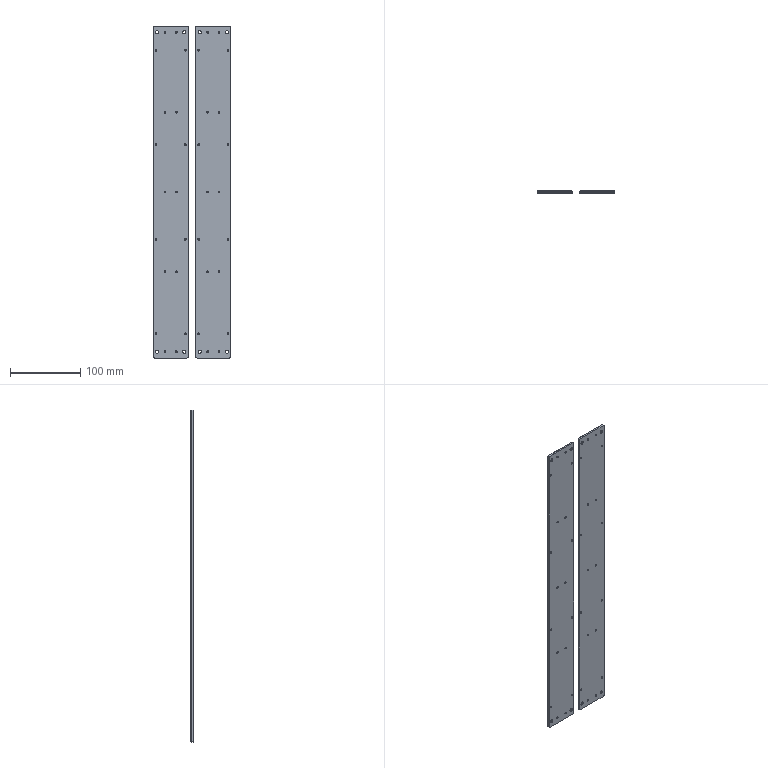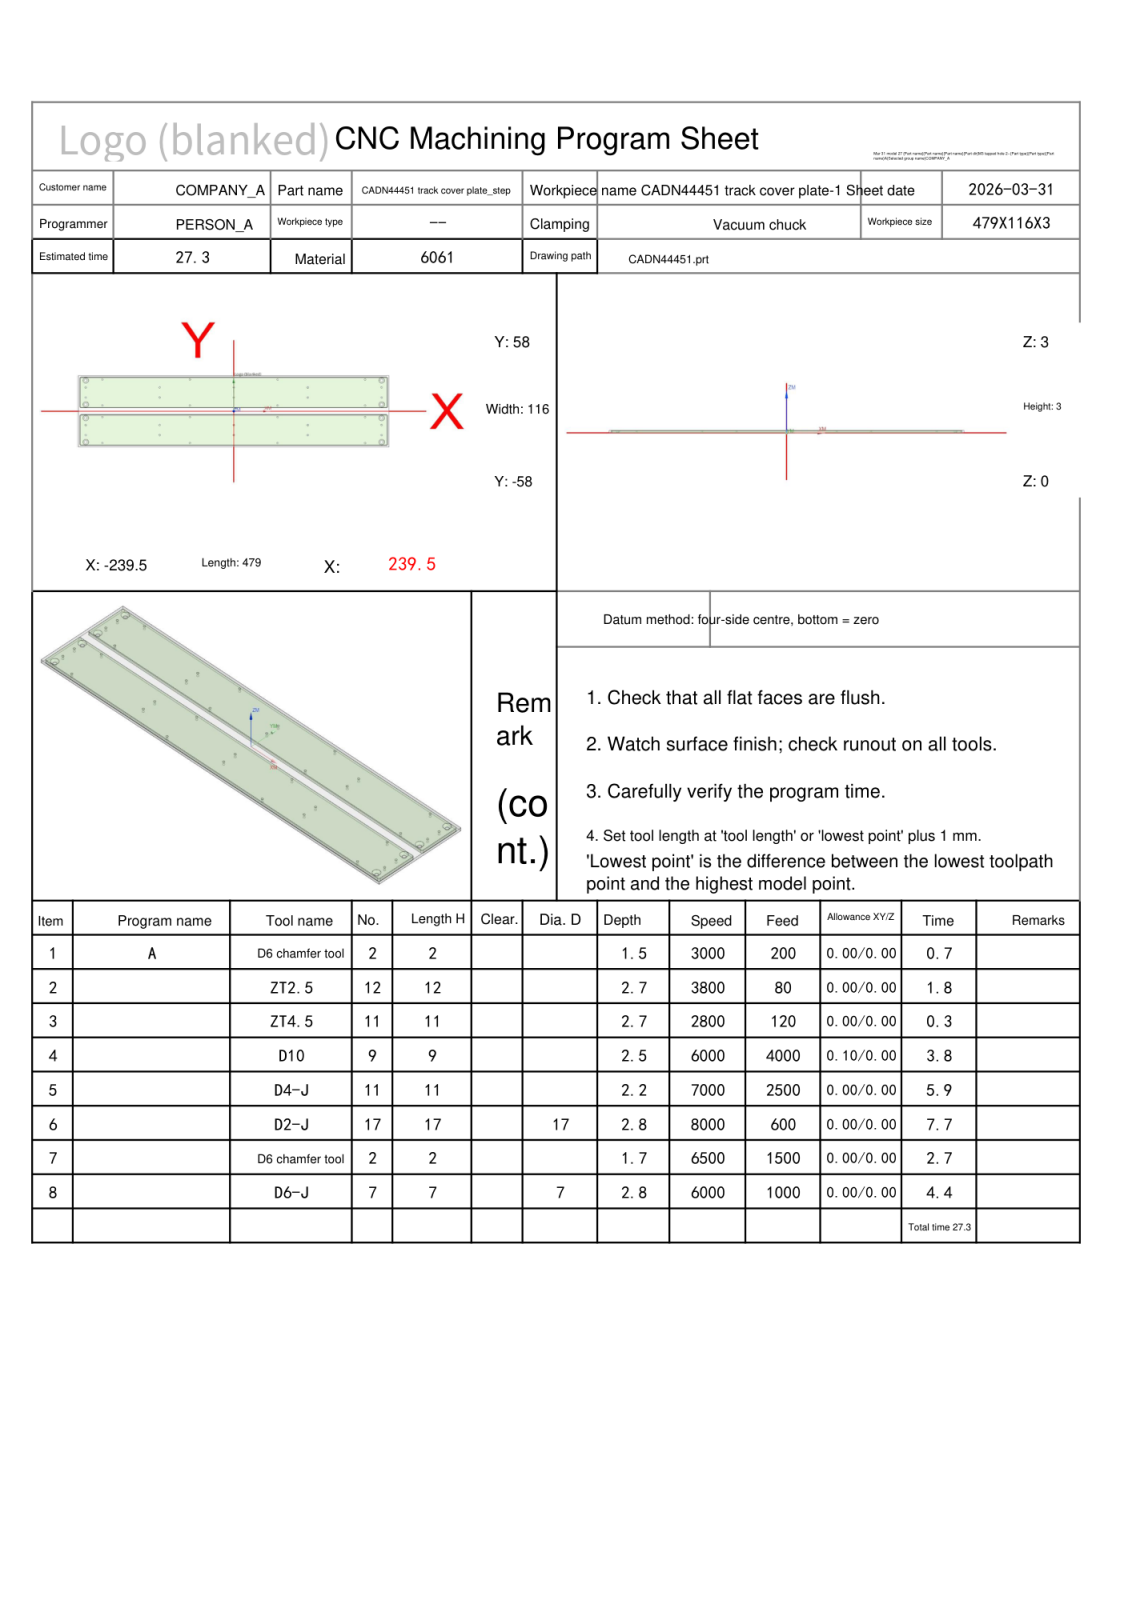NC program | NX | posted by the shop | part box 111 x 3 x 474 mm
Lines 11150 to 12144 of 17996:
N6 T17 M06
(D2-J  D=2. R=0. H=17 ce=0.00 di=0.00)
G00 G90 G54 X229.215 Y49.987 M03 S8000
G43 H17 Z23.
M08
Z1.5
G01 Y50.11 Z1.494 F600.
X229.159 Y50.381 Z1.479
X229.044 Y50.632 Z1.465
X228.875 Y50.85 Z1.45
X228.662 Y51.025 Z1.436
X228.414 Y51.148 Z1.421
X228.146 Y51.211 Z1.407
X227.89 Y51.215 Z1.393
X227.614 Y51.157 Z1.379
X227.358 Y51.038 Z1.364
X227.137 Y50.863 Z1.349
X226.962 Y50.642 Z1.334
X226.843 Y50.386 Z1.319
X226.785 Y50.11 Z1.305
Y49.89 Z1.293
X226.843 Y49.614 Z1.278
X226.962 Y49.358 Z1.264
X227.137 Y49.137 Z1.249
X227.358 Y48.962 Z1.234
X227.614 Y48.843 Z1.219
X227.89 Y48.785 Z1.204
X228.11 Z1.193
X228.386 Y48.843 Z1.178
X228.642 Y48.962 Z1.163
X228.863 Y49.137 Z1.148
X229.038 Y49.358 Z1.134
X229.157 Y49.614 Z1.119
X229.215 Y49.89 Z1.104
Y50.11 Z1.093
X229.159 Y50.381 Z1.078
X229.044 Y50.632 Z1.064
X228.875 Y50.85 Z1.049
X228.662 Y51.025 Z1.035
X228.414 Y51.148 Z1.02
X228.146 Y51.211 Z1.006
X228.035 Y51.215 Z1.
G41 D17
X228. Y51.25
G03 X226.75 Y50. Z.958 I0.0 J-1.25
X228. Y48.75 Z.915 I1.25 J0.0
X229.25 Y50. Z.873 I0.0 J1.25
X228. Y51.25 Z.83 I-1.25 J0.0
X226.75 Y50. Z.788 I0.0 J-1.25
X228. Y48.75 Z.745 I1.25 J0.0
X229.25 Y50. Z.703 I0.0 J1.25
X228. Y51.25 Z.66 I-1.25 J0.0
X226.75 Y50. Z.618 I0.0 J-1.25
X228. Y48.75 Z.575 I1.25 J0.0
X229.25 Y50. Z.533 I0.0 J1.25
X228. Y51.25 Z.49 I-1.25 J0.0
X226.75 Y50. Z.448 I0.0 J-1.25
X228. Y48.75 Z.405 I1.25 J0.0
X229.25 Y50. Z.363 I0.0 J1.25
X228. Y51.25 Z.32 I-1.25 J0.0
X226.75 Y50. Z.278 I0.0 J-1.25
X228. Y48.75 Z.235 I1.25 J0.0
X229.25 Y50. Z.193 I0.0 J1.25
X228. Y51.25 Z.15 I-1.25 J0.0
X226.75 Y50. I0.0 J-1.25
X228. Y48.75 I1.25 J0.0
X229.25 Y50. I0.0 J1.25
X228. Y51.25 I-1.25 J0.0
X227.607 Y51.187 I0.0 J-1.25
G01 X227.581 Y51.176
X227.569 Y51.15
X227.575 Y51.123
G40 X227.591 Y51.076
Z1.15
G00 Z23.
X227.987 Y9.785
Z1.5
G01 X228.11 Z1.494
X228.381 Y9.841 Z1.479
X228.632 Y9.956 Z1.465
X228.85 Y10.125 Z1.45
X229.025 Y10.338 Z1.436
X229.148 Y10.586 Z1.421
X229.211 Y10.854 Z1.407
X229.215 Y11.11 Z1.393
X229.157 Y11.386 Z1.379
X229.038 Y11.642 Z1.364
X228.863 Y11.863 Z1.349
X228.642 Y12.038 Z1.334
X228.386 Y12.157 Z1.319
X228.11 Y12.215 Z1.305
X227.89 Z1.293
X227.614 Y12.157 Z1.278
X227.358 Y12.038 Z1.264
X227.137 Y11.863 Z1.249
X226.962 Y11.642 Z1.234
X226.843 Y11.386 Z1.219
X226.785 Y11.11 Z1.204
Y10.89 Z1.193
X226.843 Y10.614 Z1.178
X226.962 Y10.358 Z1.163
X227.137 Y10.137 Z1.148
X227.358 Y9.962 Z1.134
X227.614 Y9.843 Z1.119
X227.89 Y9.785 Z1.104
X228.11 Z1.093
X228.381 Y9.841 Z1.078
X228.632 Y9.956 Z1.064
X228.85 Y10.125 Z1.049
X229.025 Y10.338 Z1.035
X229.148 Y10.586 Z1.02
X229.211 Y10.854 Z1.006
X229.215 Y10.965 Z1.
G41 D17
X229.25 Y11.
G03 X228. Y12.25 Z.958 I-1.25 J0.0
X226.75 Y11. Z.915 I0.0 J-1.25
X228. Y9.75 Z.873 I1.25 J0.0
X229.25 Y11. Z.83 I0.0 J1.25
X228. Y12.25 Z.788 I-1.25 J0.0
X226.75 Y11. Z.745 I0.0 J-1.25
X228. Y9.75 Z.703 I1.25 J0.0
X229.25 Y11. Z.66 I0.0 J1.25
X228. Y12.25 Z.618 I-1.25 J0.0
X226.75 Y11. Z.575 I0.0 J-1.25
X228. Y9.75 Z.533 I1.25 J0.0
X229.25 Y11. Z.49 I0.0 J1.25
X228. Y12.25 Z.448 I-1.25 J0.0
X226.75 Y11. Z.405 I0.0 J-1.25
X228. Y9.75 Z.363 I1.25 J0.0
X229.25 Y11. Z.32 I0.0 J1.25
X228. Y12.25 Z.278 I-1.25 J0.0
X226.75 Y11. Z.235 I0.0 J-1.25
X228. Y9.75 Z.193 I1.25 J0.0
X229.25 Y11. Z.15 I0.0 J1.25
X228. Y12.25 I-1.25 J0.0
X226.75 Y11. I0.0 J-1.25
X228. Y9.75 I1.25 J0.0
X229.25 Y11. I0.0 J1.25
X229.187 Y11.393 I-1.25 J0.0
G01 X229.176 Y11.419
X229.15 Y11.431
X229.123 Y11.425
G40 X229.076 Y11.409
Z1.15
G00 Z23.
X227.987 Y-12.215
Z1.5
G01 X228.11 Z1.494
X228.381 Y-12.159 Z1.479
X228.632 Y-12.044 Z1.465
X228.85 Y-11.875 Z1.45
X229.025 Y-11.662 Z1.436
X229.148 Y-11.414 Z1.421
X229.211 Y-11.146 Z1.407
X229.215 Y-10.89 Z1.393
X229.157 Y-10.614 Z1.379
X229.038 Y-10.358 Z1.364
X228.863 Y-10.137 Z1.349
X228.642 Y-9.962 Z1.334
X228.386 Y-9.843 Z1.319
X228.11 Y-9.785 Z1.305
X227.89 Z1.293
X227.614 Y-9.843 Z1.278
X227.358 Y-9.962 Z1.264
X227.137 Y-10.137 Z1.249
X226.962 Y-10.358 Z1.234
X226.843 Y-10.614 Z1.219
X226.785 Y-10.89 Z1.204
Y-11.11 Z1.193
X226.843 Y-11.386 Z1.178
X226.962 Y-11.642 Z1.163
X227.137 Y-11.863 Z1.148
X227.358 Y-12.038 Z1.134
X227.614 Y-12.157 Z1.119
X227.89 Y-12.215 Z1.104
X228.11 Z1.093
X228.381 Y-12.159 Z1.078
X228.632 Y-12.044 Z1.064
X228.85 Y-11.875 Z1.049
X229.025 Y-11.662 Z1.035
X229.148 Y-11.414 Z1.02
X229.211 Y-11.146 Z1.006
X229.215 Y-11.035 Z1.
G41 D17
X229.25 Y-11.
G03 X228. Y-9.75 Z.958 I-1.25 J0.0
X226.75 Y-11. Z.915 I0.0 J-1.25
X228. Y-12.25 Z.873 I1.25 J0.0
X229.25 Y-11. Z.83 I0.0 J1.25
X228. Y-9.75 Z.788 I-1.25 J0.0
X226.75 Y-11. Z.745 I0.0 J-1.25
X228. Y-12.25 Z.703 I1.25 J0.0
X229.25 Y-11. Z.66 I0.0 J1.25
X228. Y-9.75 Z.618 I-1.25 J0.0
X226.75 Y-11. Z.575 I0.0 J-1.25
X228. Y-12.25 Z.533 I1.25 J0.0
X229.25 Y-11. Z.49 I0.0 J1.25
X228. Y-9.75 Z.448 I-1.25 J0.0
X226.75 Y-11. Z.405 I0.0 J-1.25
X228. Y-12.25 Z.363 I1.25 J0.0
X229.25 Y-11. Z.32 I0.0 J1.25
X228. Y-9.75 Z.278 I-1.25 J0.0
X226.75 Y-11. Z.235 I0.0 J-1.25
X228. Y-12.25 Z.193 I1.25 J0.0
X229.25 Y-11. Z.15 I0.0 J1.25
X228. Y-9.75 I-1.25 J0.0
X226.75 Y-11. I0.0 J-1.25
X228. Y-12.25 I1.25 J0.0
X229.25 Y-11. I0.0 J1.25
X229.187 Y-10.607 I-1.25 J0.0
G01 X229.176 Y-10.581
X229.15 Y-10.569
X229.123 Y-10.575
G40 X229.076 Y-10.591
Z1.15
G00 Z23.
X226.785 Y-49.987
Z1.5
G01 Y-50.11 Z1.494
X226.841 Y-50.381 Z1.479
X226.956 Y-50.632 Z1.465
X227.125 Y-50.85 Z1.45
X227.338 Y-51.025 Z1.436
X227.586 Y-51.148 Z1.421
X227.854 Y-51.211 Z1.407
X228.11 Y-51.215 Z1.393
X228.386 Y-51.157 Z1.379
X228.642 Y-51.038 Z1.364
X228.863 Y-50.863 Z1.349
X229.038 Y-50.642 Z1.334
X229.157 Y-50.386 Z1.319
X229.215 Y-50.11 Z1.305
Y-49.89 Z1.293
X229.157 Y-49.614 Z1.278
X229.038 Y-49.358 Z1.264
X228.863 Y-49.137 Z1.249
X228.642 Y-48.962 Z1.234
X228.386 Y-48.843 Z1.219
X228.11 Y-48.785 Z1.204
X227.89 Z1.193
X227.614 Y-48.843 Z1.178
X227.358 Y-48.962 Z1.163
X227.137 Y-49.137 Z1.148
X226.962 Y-49.358 Z1.134
X226.843 Y-49.614 Z1.119
X226.785 Y-49.89 Z1.104
Y-50.11 Z1.093
X226.841 Y-50.381 Z1.078
X226.956 Y-50.632 Z1.064
X227.125 Y-50.85 Z1.049
X227.338 Y-51.025 Z1.035
X227.586 Y-51.148 Z1.02
X227.854 Y-51.211 Z1.006
X227.965 Y-51.215 Z1.
G41 D17
X228. Y-51.25
G03 X229.25 Y-50. Z.958 I0.0 J1.25
X228. Y-48.75 Z.915 I-1.25 J0.0
X226.75 Y-50. Z.873 I0.0 J-1.25
X228. Y-51.25 Z.83 I1.25 J0.0
X229.25 Y-50. Z.788 I0.0 J1.25
X228. Y-48.75 Z.745 I-1.25 J0.0
X226.75 Y-50. Z.703 I0.0 J-1.25
X228. Y-51.25 Z.66 I1.25 J0.0
X229.25 Y-50. Z.618 I0.0 J1.25
X228. Y-48.75 Z.575 I-1.25 J0.0
X226.75 Y-50. Z.533 I0.0 J-1.25
X228. Y-51.25 Z.49 I1.25 J0.0
X229.25 Y-50. Z.448 I0.0 J1.25
X228. Y-48.75 Z.405 I-1.25 J0.0
X226.75 Y-50. Z.363 I0.0 J-1.25
X228. Y-51.25 Z.32 I1.25 J0.0
X229.25 Y-50. Z.278 I0.0 J1.25
X228. Y-48.75 Z.235 I-1.25 J0.0
X226.75 Y-50. Z.193 I0.0 J-1.25
X228. Y-51.25 Z.15 I1.25 J0.0
X229.25 Y-50. I0.0 J1.25
X228. Y-48.75 I-1.25 J0.0
X226.75 Y-50. I0.0 J-1.25
X228. Y-51.25 I1.25 J0.0
X228.393 Y-51.187 I0.0 J1.25
G01 X228.419 Y-51.176
X228.431 Y-51.15
X228.425 Y-51.123
G40 X228.409 Y-51.076
Z1.15
G00 Z23.
X-229.215 Y-49.987
Z1.5
G01 Y-50.11 Z1.494
X-229.159 Y-50.381 Z1.479
X-229.044 Y-50.632 Z1.465
X-228.875 Y-50.85 Z1.45
X-228.662 Y-51.025 Z1.436
X-228.414 Y-51.148 Z1.421
X-228.146 Y-51.211 Z1.407
X-227.89 Y-51.215 Z1.393
X-227.614 Y-51.157 Z1.379
X-227.358 Y-51.038 Z1.364
X-227.137 Y-50.863 Z1.349
X-226.962 Y-50.642 Z1.334
X-226.843 Y-50.386 Z1.319
X-226.785 Y-50.11 Z1.305
Y-49.89 Z1.293
X-226.843 Y-49.614 Z1.278
X-226.962 Y-49.358 Z1.264
X-227.137 Y-49.137 Z1.249
X-227.358 Y-48.962 Z1.234
X-227.614 Y-48.843 Z1.219
X-227.89 Y-48.785 Z1.204
X-228.11 Z1.193
X-228.386 Y-48.843 Z1.178
X-228.642 Y-48.962 Z1.163
X-228.863 Y-49.137 Z1.148
X-229.038 Y-49.358 Z1.134
X-229.157 Y-49.614 Z1.119
X-229.215 Y-49.89 Z1.104
Y-50.11 Z1.093
X-229.159 Y-50.381 Z1.078
X-229.044 Y-50.632 Z1.064
X-228.875 Y-50.85 Z1.049
X-228.662 Y-51.025 Z1.035
X-228.414 Y-51.148 Z1.02
X-228.146 Y-51.211 Z1.006
X-228.035 Y-51.215 Z1.
G41 D17
X-228. Y-51.25
G03 X-226.75 Y-50. Z.958 I0.0 J1.25
X-228. Y-48.75 Z.915 I-1.25 J0.0
X-229.25 Y-50. Z.873 I0.0 J-1.25
X-228. Y-51.25 Z.83 I1.25 J0.0
X-226.75 Y-50. Z.788 I0.0 J1.25
X-228. Y-48.75 Z.745 I-1.25 J0.0
X-229.25 Y-50. Z.703 I0.0 J-1.25
X-228. Y-51.25 Z.66 I1.25 J0.0
X-226.75 Y-50. Z.618 I0.0 J1.25
X-228. Y-48.75 Z.575 I-1.25 J0.0
X-229.25 Y-50. Z.533 I0.0 J-1.25
X-228. Y-51.25 Z.49 I1.25 J0.0
X-226.75 Y-50. Z.448 I0.0 J1.25
X-228. Y-48.75 Z.405 I-1.25 J0.0
X-229.25 Y-50. Z.363 I0.0 J-1.25
X-228. Y-51.25 Z.32 I1.25 J0.0
X-226.75 Y-50. Z.278 I0.0 J1.25
X-228. Y-48.75 Z.235 I-1.25 J0.0
X-229.25 Y-50. Z.193 I0.0 J-1.25
X-228. Y-51.25 Z.15 I1.25 J0.0
X-226.75 Y-50. I0.0 J1.25
X-228. Y-48.75 I-1.25 J0.0
X-229.25 Y-50. I0.0 J-1.25
X-228. Y-51.25 I1.25 J0.0
X-227.607 Y-51.187 I0.0 J1.25
G01 X-227.581 Y-51.176
X-227.569 Y-51.15
X-227.575 Y-51.123
G40 X-227.591 Y-51.076
Z1.15
G00 Z23.
X-227.987 Y-9.785
Z1.5
G01 X-228.11 Z1.494
X-228.381 Y-9.841 Z1.479
X-228.632 Y-9.956 Z1.465
X-228.85 Y-10.125 Z1.45
X-229.025 Y-10.338 Z1.436
X-229.148 Y-10.586 Z1.421
X-229.211 Y-10.854 Z1.407
X-229.215 Y-11.11 Z1.393
X-229.157 Y-11.386 Z1.379
X-229.038 Y-11.642 Z1.364
X-228.863 Y-11.863 Z1.349
X-228.642 Y-12.038 Z1.334
X-228.386 Y-12.157 Z1.319
X-228.11 Y-12.215 Z1.305
X-227.89 Z1.293
X-227.614 Y-12.157 Z1.278
X-227.358 Y-12.038 Z1.264
X-227.137 Y-11.863 Z1.249
X-226.962 Y-11.642 Z1.234
X-226.843 Y-11.386 Z1.219
X-226.785 Y-11.11 Z1.204
Y-10.89 Z1.193
X-226.843 Y-10.614 Z1.178
X-226.962 Y-10.358 Z1.163
X-227.137 Y-10.137 Z1.148
X-227.358 Y-9.962 Z1.134
X-227.614 Y-9.843 Z1.119
X-227.89 Y-9.785 Z1.104
X-228.11 Z1.093
X-228.381 Y-9.841 Z1.078
X-228.632 Y-9.956 Z1.064
X-228.85 Y-10.125 Z1.049
X-229.025 Y-10.338 Z1.035
X-229.148 Y-10.586 Z1.02
X-229.211 Y-10.854 Z1.006
X-229.215 Y-10.965 Z1.
G41 D17
X-229.25 Y-11.
G03 X-228. Y-12.25 Z.958 I1.25 J0.0
X-226.75 Y-11. Z.915 I0.0 J1.25
X-228. Y-9.75 Z.873 I-1.25 J0.0
X-229.25 Y-11. Z.83 I0.0 J-1.25
X-228. Y-12.25 Z.788 I1.25 J0.0
X-226.75 Y-11. Z.745 I0.0 J1.25
X-228. Y-9.75 Z.703 I-1.25 J0.0
X-229.25 Y-11. Z.66 I0.0 J-1.25
X-228. Y-12.25 Z.618 I1.25 J0.0
X-226.75 Y-11. Z.575 I0.0 J1.25
X-228. Y-9.75 Z.533 I-1.25 J0.0
X-229.25 Y-11. Z.49 I0.0 J-1.25
X-228. Y-12.25 Z.448 I1.25 J0.0
X-226.75 Y-11. Z.405 I0.0 J1.25
X-228. Y-9.75 Z.363 I-1.25 J0.0
X-229.25 Y-11. Z.32 I0.0 J-1.25
X-228. Y-12.25 Z.278 I1.25 J0.0
X-226.75 Y-11. Z.235 I0.0 J1.25
X-228. Y-9.75 Z.193 I-1.25 J0.0
X-229.25 Y-11. Z.15 I0.0 J-1.25
X-228. Y-12.25 I1.25 J0.0
X-226.75 Y-11. I0.0 J1.25
X-228. Y-9.75 I-1.25 J0.0
X-229.25 Y-11. I0.0 J-1.25
X-229.187 Y-11.393 I1.25 J0.0
G01 X-229.176 Y-11.419
X-229.15 Y-11.431
X-229.123 Y-11.425
G40 X-229.076 Y-11.409
Z1.15
G00 Z23.
X-227.987 Y12.215
Z1.5
G01 X-228.11 Z1.494
X-228.381 Y12.159 Z1.479
X-228.632 Y12.044 Z1.465
X-228.85 Y11.875 Z1.45
X-229.025 Y11.662 Z1.436
X-229.148 Y11.414 Z1.421
X-229.211 Y11.146 Z1.407
X-229.215 Y10.89 Z1.393
X-229.157 Y10.614 Z1.379
X-229.038 Y10.358 Z1.364
X-228.863 Y10.137 Z1.349
X-228.642 Y9.962 Z1.334
X-228.386 Y9.843 Z1.319
X-228.11 Y9.785 Z1.305
X-227.89 Z1.293
X-227.614 Y9.843 Z1.278
X-227.358 Y9.962 Z1.264
X-227.137 Y10.137 Z1.249
X-226.962 Y10.358 Z1.234
X-226.843 Y10.614 Z1.219
X-226.785 Y10.89 Z1.204
Y11.11 Z1.193
X-226.843 Y11.386 Z1.178
X-226.962 Y11.642 Z1.163
X-227.137 Y11.863 Z1.148
X-227.358 Y12.038 Z1.134
X-227.614 Y12.157 Z1.119
X-227.89 Y12.215 Z1.104
X-228.11 Z1.093
X-228.381 Y12.159 Z1.078
X-228.632 Y12.044 Z1.064
X-228.85 Y11.875 Z1.049
X-229.025 Y11.662 Z1.035
X-229.148 Y11.414 Z1.02
X-229.211 Y11.146 Z1.006
X-229.215 Y11.035 Z1.
G41 D17
X-229.25 Y11.
G03 X-228. Y9.75 Z.958 I1.25 J0.0
X-226.75 Y11. Z.915 I0.0 J1.25
X-228. Y12.25 Z.873 I-1.25 J0.0
X-229.25 Y11. Z.83 I0.0 J-1.25
X-228. Y9.75 Z.788 I1.25 J0.0
X-226.75 Y11. Z.745 I0.0 J1.25
X-228. Y12.25 Z.703 I-1.25 J0.0
X-229.25 Y11. Z.66 I0.0 J-1.25
X-228. Y9.75 Z.618 I1.25 J0.0
X-226.75 Y11. Z.575 I0.0 J1.25
X-228. Y12.25 Z.533 I-1.25 J0.0
X-229.25 Y11. Z.49 I0.0 J-1.25
X-228. Y9.75 Z.448 I1.25 J0.0
X-226.75 Y11. Z.405 I0.0 J1.25
X-228. Y12.25 Z.363 I-1.25 J0.0
X-229.25 Y11. Z.32 I0.0 J-1.25
X-228. Y9.75 Z.278 I1.25 J0.0
X-226.75 Y11. Z.235 I0.0 J1.25
X-228. Y12.25 Z.193 I-1.25 J0.0
X-229.25 Y11. Z.15 I0.0 J-1.25
X-228. Y9.75 I1.25 J0.0
X-226.75 Y11. I0.0 J1.25
X-228. Y12.25 I-1.25 J0.0
X-229.25 Y11. I0.0 J-1.25
X-229.187 Y10.607 I1.25 J0.0
G01 X-229.176 Y10.581
X-229.15 Y10.569
X-229.123 Y10.575
G40 X-229.076 Y10.591
Z1.15
G00 Z23.
X-226.785 Y49.987
Z1.5
G01 Y50.11 Z1.494
X-226.841 Y50.381 Z1.479
X-226.956 Y50.632 Z1.465
X-227.125 Y50.85 Z1.45
X-227.338 Y51.025 Z1.436
X-227.586 Y51.148 Z1.421
X-227.854 Y51.211 Z1.407
X-228.11 Y51.215 Z1.393
X-228.386 Y51.157 Z1.379
X-228.642 Y51.038 Z1.364
X-228.863 Y50.863 Z1.349
X-229.038 Y50.642 Z1.334
X-229.157 Y50.386 Z1.319
X-229.215 Y50.11 Z1.305
Y49.89 Z1.293
X-229.157 Y49.614 Z1.278
X-229.038 Y49.358 Z1.264
X-228.863 Y49.137 Z1.249
X-228.642 Y48.962 Z1.234
X-228.386 Y48.843 Z1.219
X-228.11 Y48.785 Z1.204
X-227.89 Z1.193
X-227.614 Y48.843 Z1.178
X-227.358 Y48.962 Z1.163
X-227.137 Y49.137 Z1.148
X-226.962 Y49.358 Z1.134
X-226.843 Y49.614 Z1.119
X-226.785 Y49.89 Z1.104
Y50.11 Z1.093
X-226.841 Y50.381 Z1.078
X-226.956 Y50.632 Z1.064
X-227.125 Y50.85 Z1.049
X-227.338 Y51.025 Z1.035
X-227.586 Y51.148 Z1.02
X-227.854 Y51.211 Z1.006
X-227.965 Y51.215 Z1.
G41 D17
X-228. Y51.25
G03 X-229.25 Y50. Z.958 I0.0 J-1.25
X-228. Y48.75 Z.915 I1.25 J0.0
X-226.75 Y50. Z.873 I0.0 J1.25
X-228. Y51.25 Z.83 I-1.25 J0.0
X-229.25 Y50. Z.788 I0.0 J-1.25
X-228. Y48.75 Z.745 I1.25 J0.0
X-226.75 Y50. Z.703 I0.0 J1.25
X-228. Y51.25 Z.66 I-1.25 J0.0
X-229.25 Y50. Z.618 I0.0 J-1.25
X-228. Y48.75 Z.575 I1.25 J0.0
X-226.75 Y50. Z.533 I0.0 J1.25
X-228. Y51.25 Z.49 I-1.25 J0.0
X-229.25 Y50. Z.448 I0.0 J-1.25
X-228. Y48.75 Z.405 I1.25 J0.0
X-226.75 Y50. Z.363 I0.0 J1.25
X-228. Y51.25 Z.32 I-1.25 J0.0
X-229.25 Y50. Z.278 I0.0 J-1.25
X-228. Y48.75 Z.235 I1.25 J0.0
X-226.75 Y50. Z.193 I0.0 J1.25
X-228. Y51.25 Z.15 I-1.25 J0.0
X-229.25 Y50. I0.0 J-1.25
X-228. Y48.75 I1.25 J0.0
X-226.75 Y50. I0.0 J1.25
X-228. Y51.25 I-1.25 J0.0
X-228.393 Y51.187 I0.0 J-1.25
G01 X-228.419 Y51.176
X-228.431 Y51.15
X-228.425 Y51.123
G40 X-228.409 Y51.076
Z1.15
G00 Z23.
G00 G90 X202.408 Y51.693 M03 S8000
Z23.
Z3.5
G01 X202.343 Y51.657 Z3.496 F200.
X202.282 Y51.547 Z3.49
Y51.453 Z3.485
X202.343 Y51.343 Z3.478
X202.453 Y51.282 Z3.471
X202.547 Z3.466
X202.657 Y51.343 Z3.46
X202.718 Y51.453 Z3.453
Y51.547 Z3.448
X202.67 Y51.644 Z3.443
X202.582 Y51.707 Z3.437
X202.5 Y51.718 Z3.433
X202.453 Z3.43
X202.343 Y51.657 Z3.424
X202.282 Y51.547 Z3.417
Y51.453 Z3.412
X202.343 Y51.343 Z3.406
X202.453 Y51.282 Z3.399
X202.547 Z3.394
X202.657 Y51.343 Z3.387
X202.718 Y51.453 Z3.381
Y51.547 Z3.376
X202.67 Y51.644 Z3.37
X202.582 Y51.707 Z3.365
X202.5 Y51.718 Z3.36
X202.453 Z3.358
X202.343 Y51.657 Z3.351
X202.282 Y51.547 Z3.345
Y51.453 Z3.34
X202.343 Y51.343 Z3.333
X202.453 Y51.282 Z3.327
X202.547 Z3.322
X202.657 Y51.343 Z3.315
X202.718 Y51.453 Z3.308
Y51.547 Z3.304
X202.67 Y51.644 Z3.298
X202.582 Y51.707 Z3.292
X202.5 Y51.718 Z3.288
X202.453 Z3.285
X202.343 Y51.657 Z3.279
X202.282 Y51.547 Z3.272
Y51.453 Z3.267
X202.343 Y51.343 Z3.261
X202.453 Y51.282 Z3.254
X202.547 Z3.249
X202.657 Y51.343 Z3.243
X202.718 Y51.453 Z3.236
Y51.547 Z3.231
X202.67 Y51.644 Z3.225
X202.582 Y51.707 Z3.22
X202.5 Y51.718 Z3.215
X202.453 Z3.213
X202.343 Y51.657 Z3.206
X202.282 Y51.547 Z3.2
Y51.453 Z3.195
X202.343 Y51.343 Z3.188
X202.453 Y51.282 Z3.182
X202.547 Z3.177
X202.657 Y51.343 Z3.17
X202.718 Y51.453 Z3.164
Y51.547 Z3.159
X202.67 Y51.644 Z3.153
X202.582 Y51.707 Z3.147
X202.5 Y51.718 Z3.143
X202.453 Z3.141
X202.343 Y51.657 Z3.134
X202.282 Y51.547 Z3.127
Y51.453 Z3.122
X202.343 Y51.343 Z3.116
X202.453 Y51.282 Z3.109
X202.547 Z3.104
X202.657 Y51.343 Z3.098
X202.718 Y51.453 Z3.091
Y51.547 Z3.086
X202.67 Y51.644 Z3.081
X202.582 Y51.707 Z3.075
X202.5 Y51.718 Z3.071
X202.453 Z3.068
X202.343 Y51.657 Z3.062
X202.282 Y51.547 Z3.055
Y51.453 Z3.05
X202.343 Y51.343 Z3.043
X202.453 Y51.282 Z3.037
X202.547 Z3.032
X202.657 Y51.343 Z3.025
X202.718 Y51.453 Z3.019
Y51.547 Z3.014
X202.67 Y51.644 Z3.008
X202.582 Y51.707 Z3.002
X202.535 Y51.715 Z3.
G41 D17
X202.5 Y51.75
G03 X202.25 Y51.5 Z2.953 I0.0 J-.25
X202.5 Y51.25 Z2.905 I.25 J0.0
X202.75 Y51.5 Z2.858 I0.0 J.25
X202.5 Y51.75 Z2.81 I-.25 J0.0
X202.25 Y51.5 Z2.763 I0.0 J-.25
X202.5 Y51.25 Z2.715 I.25 J0.0
X202.75 Y51.5 Z2.668 I0.0 J.25
X202.5 Y51.75 Z2.62 I-.25 J0.0
X202.25 Y51.5 Z2.573 I0.0 J-.25
X202.5 Y51.25 Z2.525 I.25 J0.0
X202.75 Y51.5 Z2.478 I0.0 J.25
X202.5 Y51.75 Z2.43 I-.25 J0.0
X202.25 Y51.5 Z2.383 I0.0 J-.25
X202.5 Y51.25 Z2.335 I.25 J0.0
X202.75 Y51.5 Z2.288 I0.0 J.25
X202.5 Y51.75 Z2.24 I-.25 J0.0
X202.25 Y51.5 Z2.193 I0.0 J-.25
X202.5 Y51.25 Z2.145 I.25 J0.0
X202.75 Y51.5 Z2.098 I0.0 J.25
X202.5 Y51.75 Z2.05 I-.25 J0.0
X202.25 Y51.5 Z2.003 I0.0 J-.25
X202.5 Y51.25 Z1.955 I.25 J0.0
X202.75 Y51.5 Z1.908 I0.0 J.25
X202.5 Y51.75 Z1.86 I-.25 J0.0
X202.25 Y51.5 Z1.813 I0.0 J-.25
X202.5 Y51.25 Z1.765 I.25 J0.0
X202.75 Y51.5 Z1.718 I0.0 J.25
X202.5 Y51.75 Z1.67 I-.25 J0.0
X202.25 Y51.5 Z1.623 I0.0 J-.25
X202.5 Y51.25 Z1.575 I.25 J0.0
X202.75 Y51.5 Z1.528 I0.0 J.25
X202.5 Y51.75 Z1.48 I-.25 J0.0
X202.25 Y51.5 Z1.433 I0.0 J-.25
X202.5 Y51.25 Z1.385 I.25 J0.0
X202.75 Y51.5 Z1.338 I0.0 J.25
X202.5 Y51.75 Z1.29 I-.25 J0.0
X202.25 Y51.5 Z1.243 I0.0 J-.25
X202.5 Y51.25 Z1.195 I.25 J0.0
X202.75 Y51.5 Z1.148 I0.0 J.25
X202.5 Y51.75 Z1.1 I-.25 J0.0
X202.25 Y51.5 Z1.053 I0.0 J-.25
X202.5 Y51.25 Z1.005 I.25 J0.0
X202.75 Y51.5 Z.958 I0.0 J.25
X202.5 Y51.75 Z.91 I-.25 J0.0
X202.25 Y51.5 Z.863 I0.0 J-.25
X202.5 Y51.25 Z.815 I.25 J0.0
X202.75 Y51.5 Z.768 I0.0 J.25
X202.5 Y51.75 Z.72 I-.25 J0.0
X202.25 Y51.5 Z.673 I0.0 J-.25
X202.5 Y51.25 Z.625 I.25 J0.0
X202.75 Y51.5 Z.578 I0.0 J.25
X202.5 Y51.75 Z.53 I-.25 J0.0
X202.25 Y51.5 Z.483 I0.0 J-.25
X202.5 Y51.25 Z.435 I.25 J0.0
X202.75 Y51.5 Z.388 I0.0 J.25
X202.5 Y51.75 Z.34 I-.25 J0.0
X202.25 Y51.5 Z.293 I0.0 J-.25
X202.5 Y51.25 Z.245 I.25 J0.0
X202.75 Y51.5 Z.198 I0.0 J.25
X202.5 Y51.75 Z.15 I-.25 J0.0
X202.25 Y51.5 I0.0 J-.25
X202.5 Y51.25 I.25 J0.0
X202.75 Y51.5 I0.0 J.25
X202.5 Y51.75 I-.25 J0.0
X202.25 Y51.5 I0.0 J-.25
G01 Y51.493
X202.253 Y51.465
X202.274 Y51.446
X202.302 Y51.444
G40 X202.352 Y51.446
Z1.15
G00 Z23.
X228.193 Y38.692
Z3.5
G01 X228.157 Y38.757 Z3.496
X228.047 Y38.818 Z3.49
X227.953 Z3.485
X227.843 Y38.757 Z3.478
X227.782 Y38.647 Z3.471
Y38.553 Z3.466
X227.843 Y38.443 Z3.46
X227.953 Y38.382 Z3.453
X228.047 Z3.448
X228.144 Y38.43 Z3.443
X228.207 Y38.518 Z3.437
X228.218 Y38.6 Z3.433
Y38.647 Z3.43
X228.157 Y38.757 Z3.424
X228.047 Y38.818 Z3.417
X227.953 Z3.412
X227.843 Y38.757 Z3.406
X227.782 Y38.647 Z3.399
Y38.553 Z3.394
X227.843 Y38.443 Z3.387
X227.953 Y38.382 Z3.381
X228.047 Z3.376
X228.144 Y38.43 Z3.37
X228.207 Y38.518 Z3.365
X228.218 Y38.6 Z3.36
Y38.647 Z3.358
X228.157 Y38.757 Z3.351
X228.047 Y38.818 Z3.345
X227.953 Z3.34
X227.843 Y38.757 Z3.333
X227.782 Y38.647 Z3.327
Y38.553 Z3.322
X227.843 Y38.443 Z3.315
X227.953 Y38.382 Z3.308
X228.047 Z3.304
X228.144 Y38.43 Z3.298
X228.207 Y38.518 Z3.292
X228.218 Y38.6 Z3.288
Y38.647 Z3.285
X228.157 Y38.757 Z3.279
X228.047 Y38.818 Z3.272
X227.953 Z3.267
X227.843 Y38.757 Z3.261
X227.782 Y38.647 Z3.254
Y38.553 Z3.249
X227.843 Y38.443 Z3.243
X227.953 Y38.382 Z3.236
X228.047 Z3.231
X228.144 Y38.43 Z3.225
X228.207 Y38.518 Z3.22
X228.218 Y38.6 Z3.215
Y38.647 Z3.213
X228.157 Y38.757 Z3.206
X228.047 Y38.818 Z3.2
X227.953 Z3.195
X227.843 Y38.757 Z3.188
X227.782 Y38.647 Z3.182
Y38.553 Z3.177
X227.843 Y38.443 Z3.17
X227.953 Y38.382 Z3.164
X228.047 Z3.159
X228.144 Y38.43 Z3.153
X228.207 Y38.518 Z3.147
X228.218 Y38.6 Z3.143
Y38.647 Z3.141
X228.157 Y38.757 Z3.134
X228.047 Y38.818 Z3.127
X227.953 Z3.122
X227.843 Y38.757 Z3.116
X227.782 Y38.647 Z3.109
Y38.553 Z3.104
X227.843 Y38.443 Z3.098
X227.953 Y38.382 Z3.091
X228.047 Z3.086
X228.144 Y38.43 Z3.081
X228.207 Y38.518 Z3.075
X228.218 Y38.6 Z3.071
Y38.647 Z3.068
X228.157 Y38.757 Z3.062
X228.047 Y38.818 Z3.055
X227.953 Z3.05
X227.843 Y38.757 Z3.043
X227.782 Y38.647 Z3.037
Y38.553 Z3.032
X227.843 Y38.443 Z3.025
X227.953 Y38.382 Z3.019
X228.047 Z3.014
X228.144 Y38.43 Z3.008
X228.207 Y38.518 Z3.002
X228.215 Y38.565 Z3.
G41 D17
X228.25 Y38.6
G03 X228. Y38.85 Z2.953 I-.25 J0.0
X227.75 Y38.6 Z2.905 I0.0 J-.25
X228. Y38.35 Z2.858 I.25 J0.0
X228.25 Y38.6 Z2.81 I0.0 J.25
X228. Y38.85 Z2.763 I-.25 J0.0
X227.75 Y38.6 Z2.715 I0.0 J-.25
X228. Y38.35 Z2.668 I.25 J0.0
X228.25 Y38.6 Z2.62 I0.0 J.25
X228. Y38.85 Z2.573 I-.25 J0.0
X227.75 Y38.6 Z2.525 I0.0 J-.25
X228. Y38.35 Z2.478 I.25 J0.0
X228.25 Y38.6 Z2.43 I0.0 J.25
X228. Y38.85 Z2.383 I-.25 J0.0
X227.75 Y38.6 Z2.335 I0.0 J-.25
X228. Y38.35 Z2.288 I.25 J0.0
X228.25 Y38.6 Z2.24 I0.0 J.25
X228. Y38.85 Z2.193 I-.25 J0.0
X227.75 Y38.6 Z2.145 I0.0 J-.25
X228. Y38.35 Z2.098 I.25 J0.0
X228.25 Y38.6 Z2.05 I0.0 J.25
X228. Y38.85 Z2.003 I-.25 J0.0
X227.75 Y38.6 Z1.955 I0.0 J-.25
X228. Y38.35 Z1.908 I.25 J0.0
X228.25 Y38.6 Z1.86 I0.0 J.25
X228. Y38.85 Z1.813 I-.25 J0.0
X227.75 Y38.6 Z1.765 I0.0 J-.25
X228. Y38.35 Z1.718 I.25 J0.0
X228.25 Y38.6 Z1.67 I0.0 J.25
X228. Y38.85 Z1.623 I-.25 J0.0
X227.75 Y38.6 Z1.575 I0.0 J-.25
X228. Y38.35 Z1.528 I.25 J0.0
X228.25 Y38.6 Z1.48 I0.0 J.25
X228. Y38.85 Z1.433 I-.25 J0.0
X227.75 Y38.6 Z1.385 I0.0 J-.25
X228. Y38.35 Z1.338 I.25 J0.0
X228.25 Y38.6 Z1.29 I0.0 J.25
X228. Y38.85 Z1.243 I-.25 J0.0
X227.75 Y38.6 Z1.195 I0.0 J-.25
X228. Y38.35 Z1.148 I.25 J0.0
X228.25 Y38.6 Z1.1 I0.0 J.25
X228. Y38.85 Z1.053 I-.25 J0.0
X227.75 Y38.6 Z1.005 I0.0 J-.25
X228. Y38.35 Z.958 I.25 J0.0
X228.25 Y38.6 Z.91 I0.0 J.25
X228. Y38.85 Z.863 I-.25 J0.0
X227.75 Y38.6 Z.815 I0.0 J-.25
X228. Y38.35 Z.768 I.25 J0.0
X228.25 Y38.6 Z.72 I0.0 J.25
X228. Y38.85 Z.673 I-.25 J0.0
X227.75 Y38.6 Z.625 I0.0 J-.25
X228. Y38.35 Z.578 I.25 J0.0
X228.25 Y38.6 Z.53 I0.0 J.25
X228. Y38.85 Z.483 I-.25 J0.0
X227.75 Y38.6 Z.435 I0.0 J-.25
X228. Y38.35 Z.388 I.25 J0.0
X228.25 Y38.6 Z.34 I0.0 J.25
X228. Y38.85 Z.293 I-.25 J0.0
X227.75 Y38.6 Z.245 I0.0 J-.25
X228. Y38.35 Z.198 I.25 J0.0
X228.25 Y38.6 Z.15 I0.0 J.25
X228. Y38.85 I-.25 J0.0
X227.75 Y38.6 I0.0 J-.25
X228. Y38.35 I.25 J0.0
X228.25 Y38.6 I0.0 J.25
X228. Y38.85 I-.25 J0.0
G01 X227.993
X227.965 Y38.847
X227.946 Y38.826
X227.944 Y38.798
G40 X227.946 Y38.748
Z1.15
G00 Z23.
X228.193 Y22.492
Z3.5
G01 X228.157 Y22.557 Z3.496
X228.047 Y22.618 Z3.49
X227.953 Z3.485
X227.843 Y22.557 Z3.478
X227.782 Y22.447 Z3.471
Y22.353 Z3.466
X227.843 Y22.243 Z3.46
X227.953 Y22.182 Z3.453
X228.047 Z3.448
X228.144 Y22.23 Z3.443
X228.207 Y22.318 Z3.437
X228.218 Y22.4 Z3.433
Y22.447 Z3.43
X228.157 Y22.557 Z3.424
X228.047 Y22.618 Z3.417
X227.953 Z3.412
X227.843 Y22.557 Z3.406
X227.782 Y22.447 Z3.399
Y22.353 Z3.394
X227.843 Y22.243 Z3.387
X227.953 Y22.182 Z3.381
X228.047 Z3.376
X228.144 Y22.23 Z3.37
X228.207 Y22.318 Z3.365
X228.218 Y22.4 Z3.36
Y22.447 Z3.358
X228.157 Y22.557 Z3.351
X228.047 Y22.618 Z3.345
X227.953 Z3.34
X227.843 Y22.557 Z3.333
X227.782 Y22.447 Z3.327
Y22.353 Z3.322
X227.843 Y22.243 Z3.315
X227.953 Y22.182 Z3.308
X228.047 Z3.304
X228.144 Y22.23 Z3.298
X228.207 Y22.318 Z3.292
X228.218 Y22.4 Z3.288
Y22.447 Z3.285
X228.157 Y22.557 Z3.279
X228.047 Y22.618 Z3.272
X227.953 Z3.267
X227.843 Y22.557 Z3.261
X227.782 Y22.447 Z3.254
Y22.353 Z3.249
X227.843 Y22.243 Z3.243
X227.953 Y22.182 Z3.236
X228.047 Z3.231
X228.144 Y22.23 Z3.225
X228.207 Y22.318 Z3.22
X228.218 Y22.4 Z3.215
Y22.447 Z3.213
X228.157 Y22.557 Z3.206
X228.047 Y22.618 Z3.2
X227.953 Z3.195
X227.843 Y22.557 Z3.188
X227.782 Y22.447 Z3.182
Y22.353 Z3.177
X227.843 Y22.243 Z3.17
X227.953 Y22.182 Z3.164
X228.047 Z3.159
X228.144 Y22.23 Z3.153
X228.207 Y22.318 Z3.147
X228.218 Y22.4 Z3.143
Y22.447 Z3.141
X228.157 Y22.557 Z3.134
X228.047 Y22.618 Z3.127
X227.953 Z3.122
X227.843 Y22.557 Z3.116
X227.782 Y22.447 Z3.109
Y22.353 Z3.104
X227.843 Y22.243 Z3.098
X227.953 Y22.182 Z3.091
X228.047 Z3.086
X228.144 Y22.23 Z3.081
X228.207 Y22.318 Z3.075
X228.218 Y22.4 Z3.071
Y22.447 Z3.068
X228.157 Y22.557 Z3.062
X228.047 Y22.618 Z3.055
X227.953 Z3.05
X227.843 Y22.557 Z3.043
X227.782 Y22.447 Z3.037
Y22.353 Z3.032
X227.843 Y22.243 Z3.025
X227.953 Y22.182 Z3.019
X228.047 Z3.014
X228.144 Y22.23 Z3.008